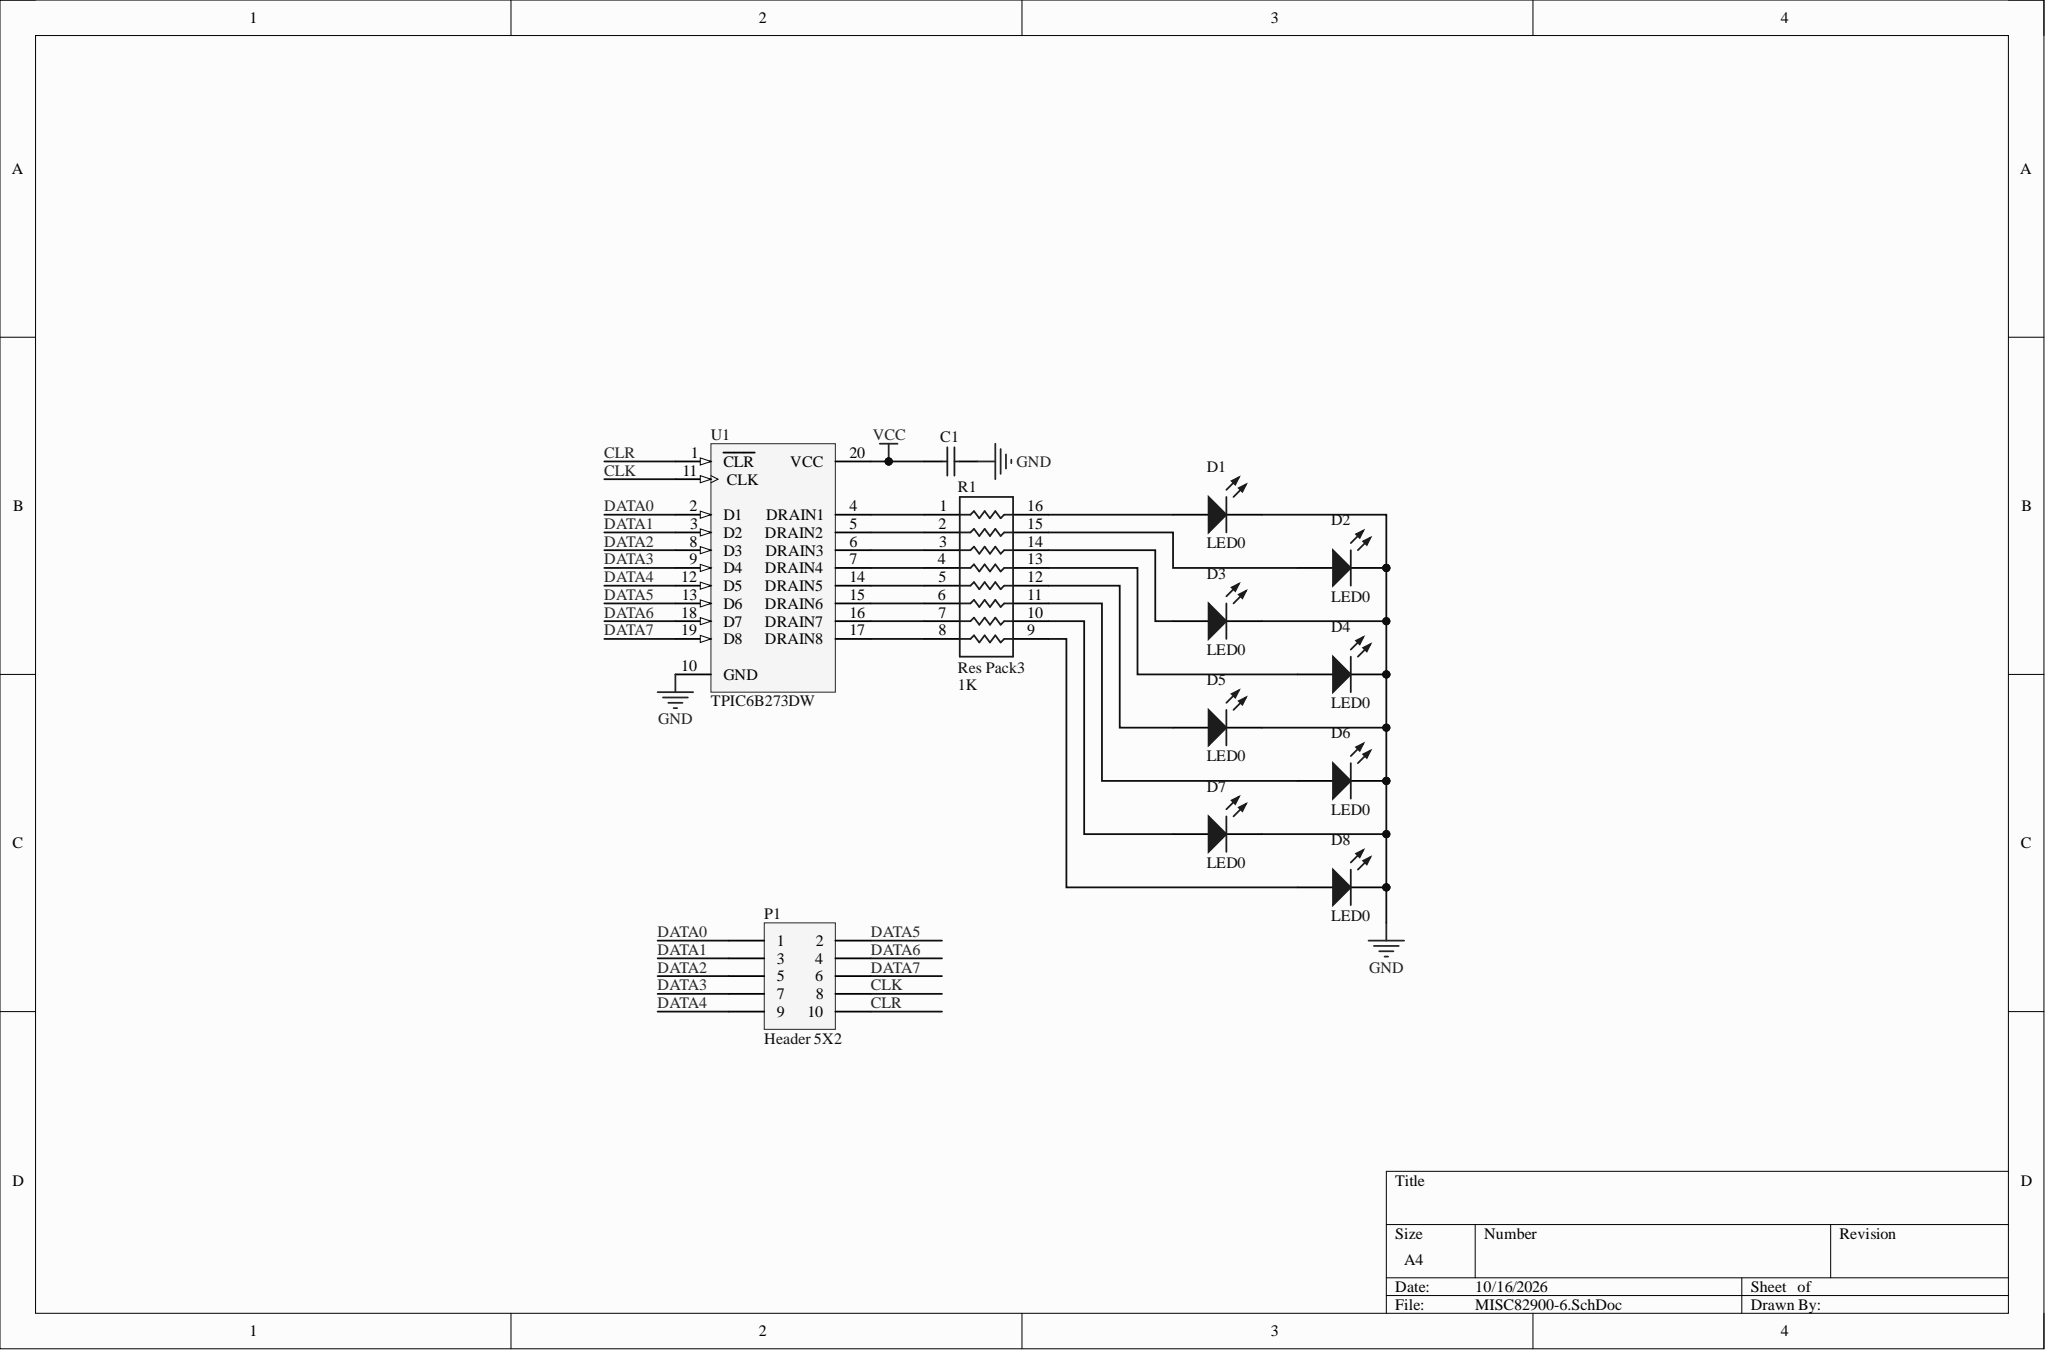Circuit board | Altium Designer | 12 parts | 28 nets
Bill of materials:
Comment,Description,Designator,Footprint,LibRef,Quantity
"Cap","Capacitor","C1","RAD-0.3","Cap","1"
"LED0","Typical INFRARED GaAs LED","D1, D2, D3, D4, D5, D6, D7, D8","LED-0","LED0","8"
"Header 5X2","Header, 5-Pin, Dual row","P1","HDR2X5","Header 5X2","1"
"Res Pack3","Isolated Resistor Network","R1","SO-16_N","Res Pack3","1"
"TPIC6B273DW","Power Logic Octal D-Type Latch","U1","DW020","TPIC6B273DW","1"
Netlist (Protel format):
[
C1
RAD-0.3
Cap



]
[
D1
LED-0
LED0



]
[
D2
LED-0
LED0



]
[
D3
LED-0
LED0



]
[
D4
LED-0
LED0



]
[
D5
LED-0
LED0



]
[
D6
LED-0
LED0



]
[
D7
LED-0
LED0



]
[
D8
LED-0
LED0



]
[
P1
HDR2X5
Header 5X2



]
[
R1
SO-16_N
Res Pack3



]
[
U1
DW020
TPIC6B273DW



]
(
VCC
C1-1
U1-20
)
(
NetR1_8
R1-8
U1-17
)
(
NetR1_7
R1-7
U1-16
)
(
NetR1_6
R1-6
U1-15
)
(
NetR1_5
R1-5
U1-14
)
(
NetR1_4
R1-4
U1-7
)
(
NetR1_3
R1-3
U1-6
)
(
NetR1_2
R1-2
U1-5
)
(
NetR1_1
R1-1
U1-4
)
(
NetD8_1
D8-1
R1-9
)
(
NetD7_1
D7-1
R1-10
)
(
NetD6_1
D6-1
R1-11
)
(
NetD5_1
D5-1
R1-12
)
(
NetD4_1
D4-1
R1-13
)
(
NetD3_1
D3-1
R1-14
)
(
NetD2_1
D2-1
R1-15
)
(
NetD1_1
D1-1
R1-16
)
(
GND
C1-2
D1-2
D2-2
D3-2
D4-2
D5-2
D6-2
D7-2
D8-2
U1-10
)
(
DATA7
P1-6
U1-19
)
(
DATA6
P1-4
U1-18
)
(
DATA5
P1-2
U1-13
)
(
DATA4
P1-9
U1-12
)
(
DATA3
P1-7
U1-9
)
(
DATA2
P1-5
U1-8
)
(
DATA1
P1-3
U1-3
)
(
DATA0
P1-1
U1-2
)
(
CLR
P1-10
U1-1
)
(
CLK
P1-8
U1-11
)